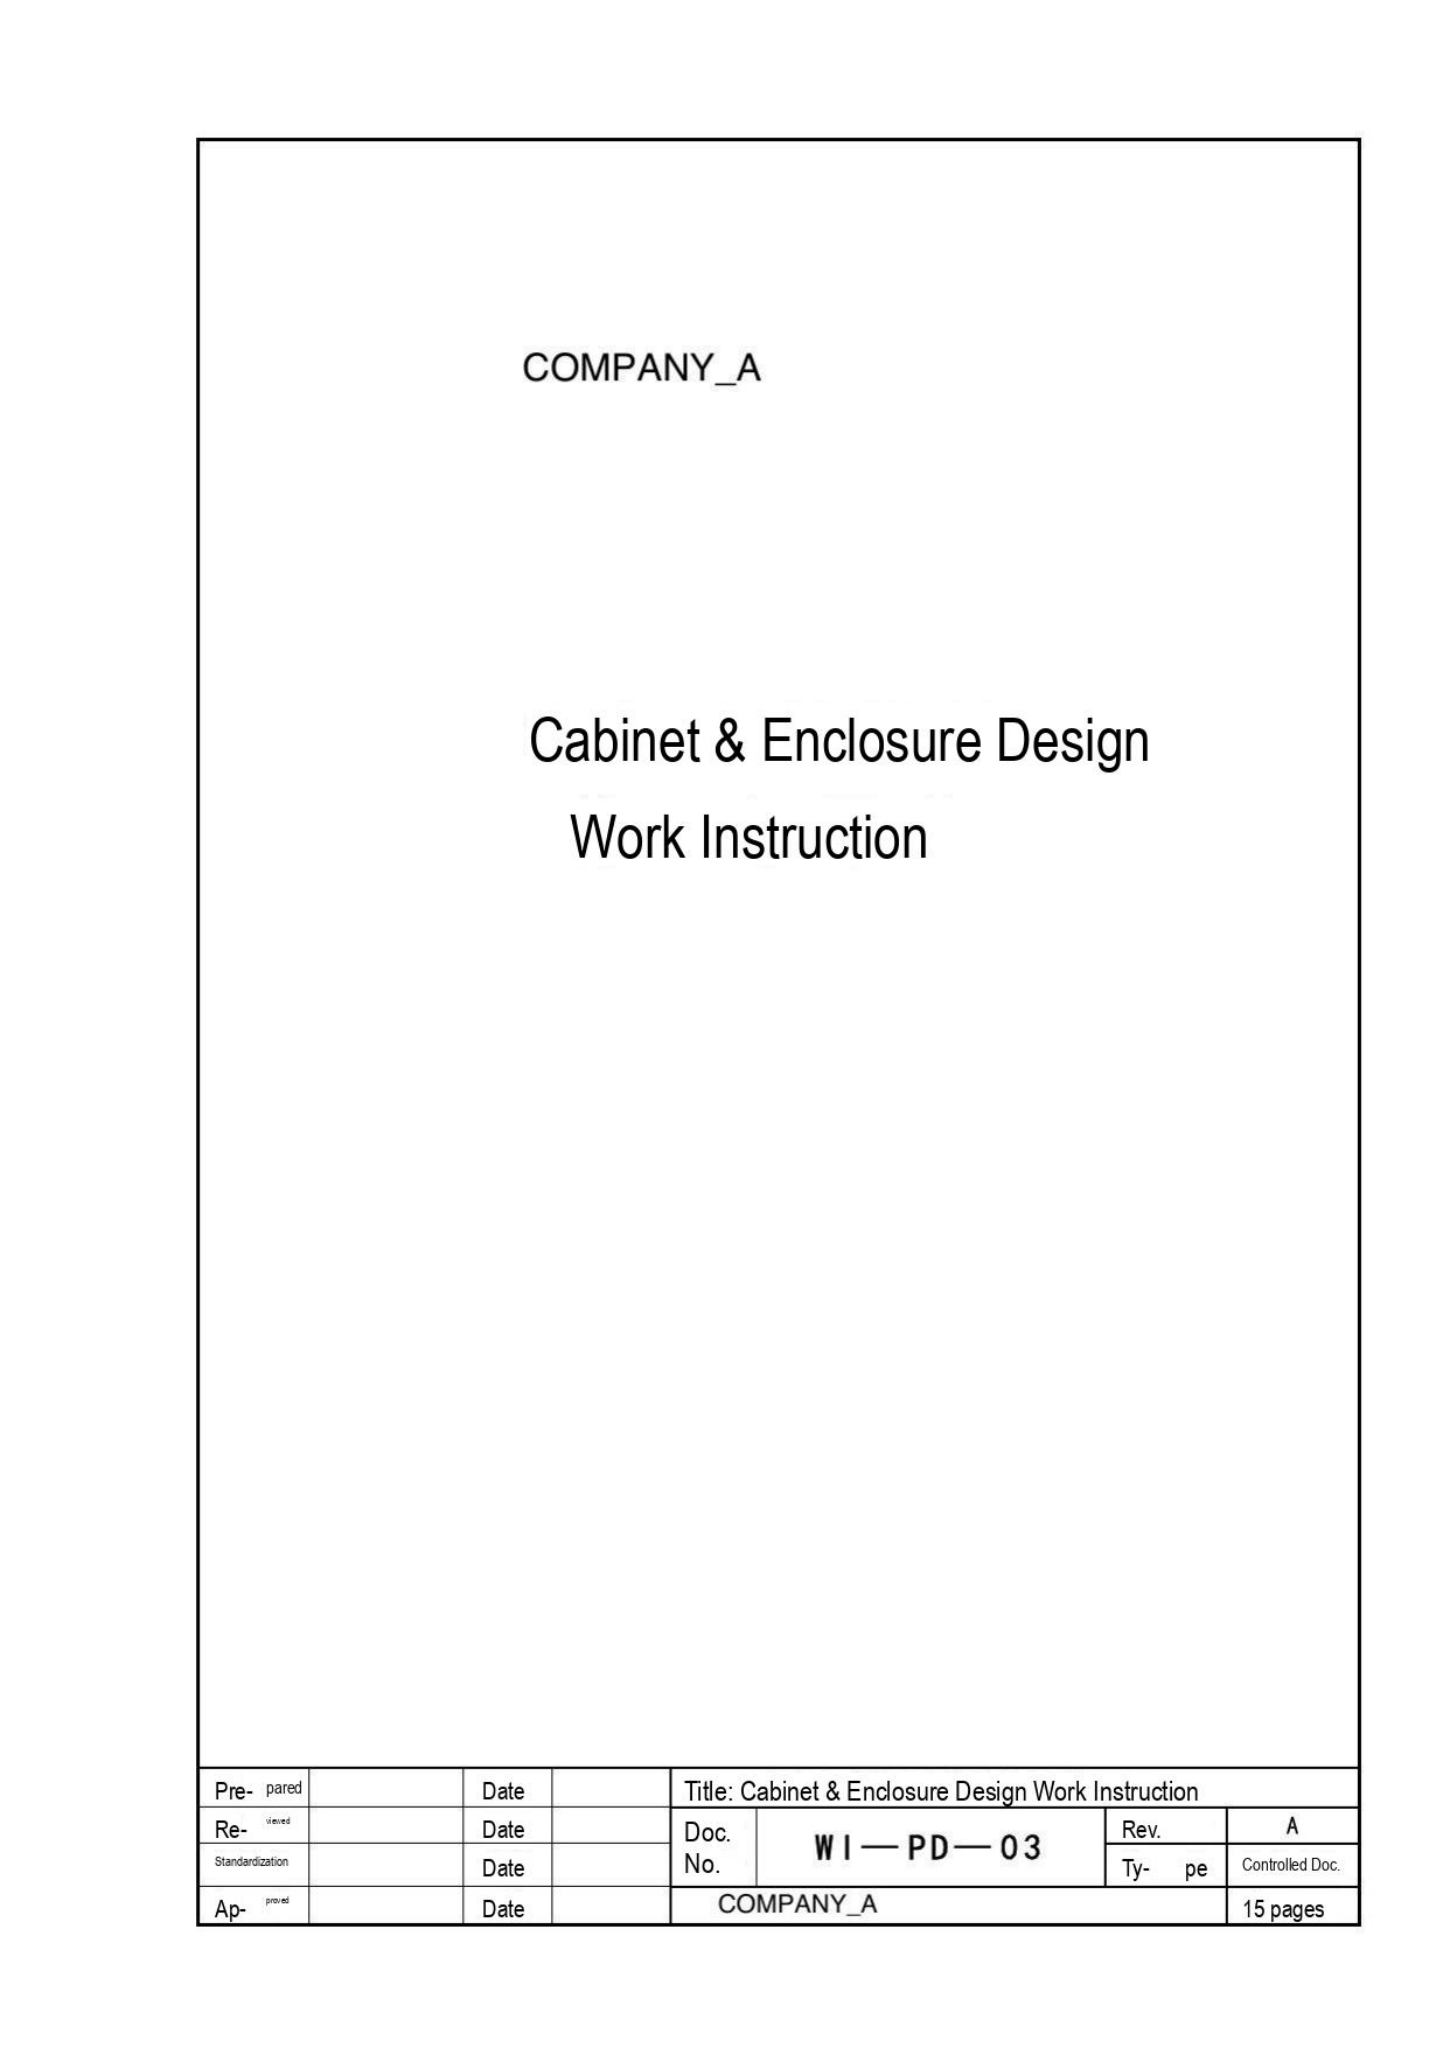COMPANY_A

Cabinet & Enclosure Design

Work Instruction

| Pre- pared | | Date | | Title: Cabinet & Enclosure Design Work Instruction | | | |
|---|---|---|---|---|---|---|---|
| Re- viewed | | Date | | Doc. No. | WI—PD—03 | Rev. | A |
| Standardization | | Date | | | | Ty- pe | Controlled Doc. |
| Ap- proved | | Date | | COMPANY_A | | | 15 pages |
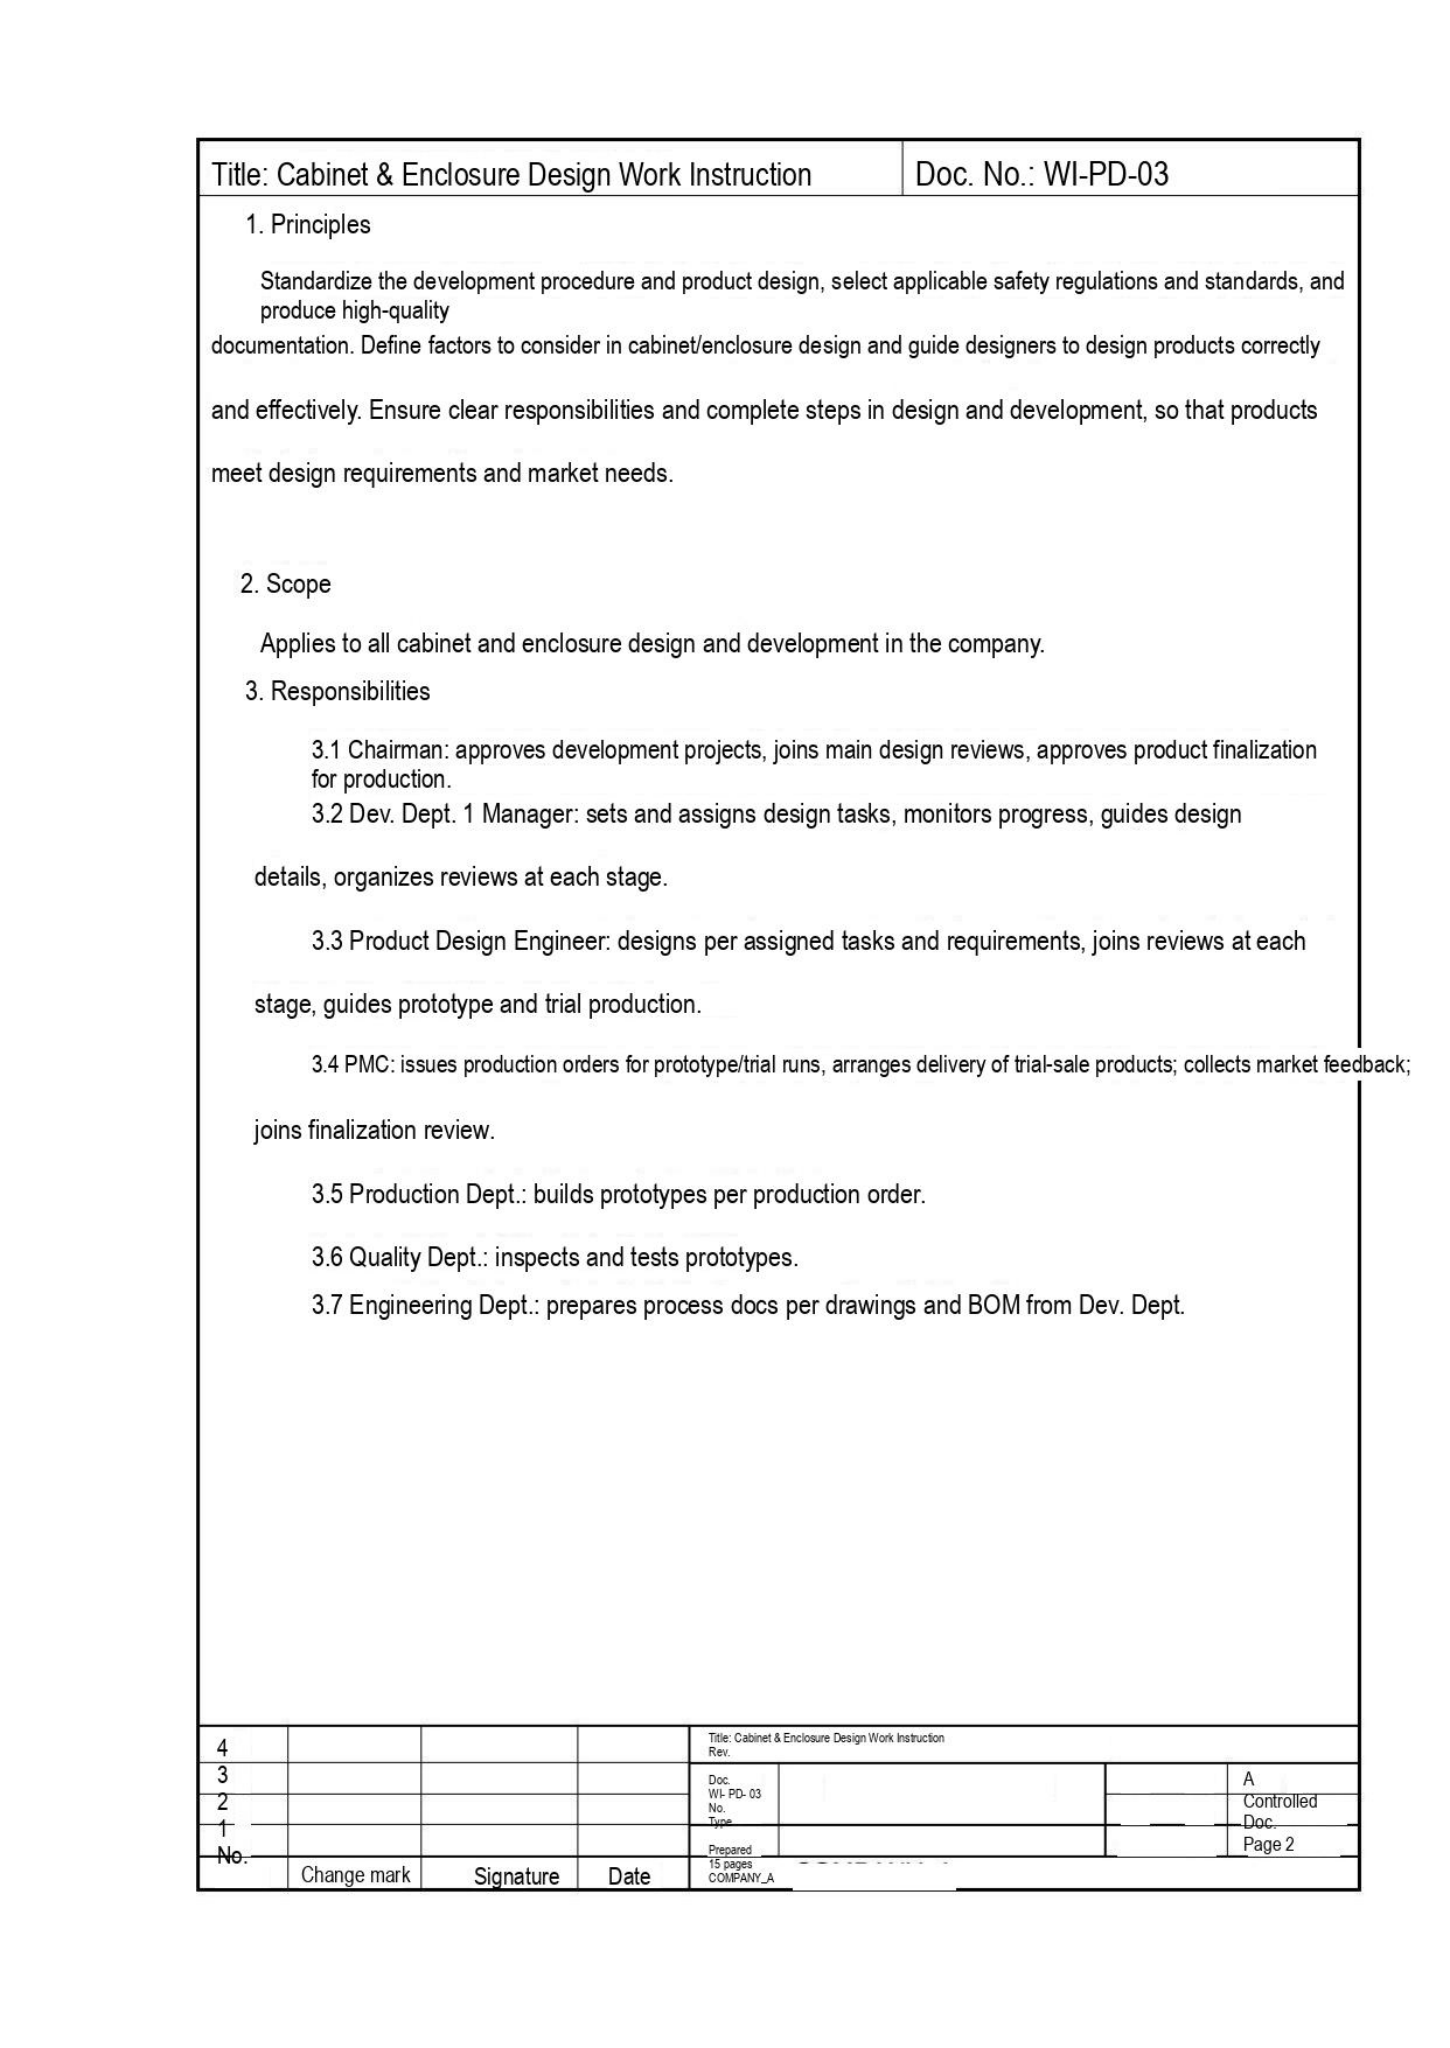Title: Cabinet & Enclosure Design Work Instruction | Doc. No.: WI-PD-03

1. Principles

Standardize the development procedure and product design, select applicable safety regulations and standards, and produce high-quality documentation. Define factors to consider in cabinet/enclosure design and guide designers to design products correctly and effectively. Ensure clear responsibilities and complete steps in design and development, so that products meet design requirements and market needs.

2. Scope

Applies to all cabinet and enclosure design and development in the company.

3. Responsibilities

3.1 Chairman: approves development projects, joins main design reviews, approves product finalization for production.

3.2 Dev. Dept. 1 Manager: sets and assigns design tasks, monitors progress, guides design details, organizes reviews at each stage.

3.3 Product Design Engineer: designs per assigned tasks and requirements, joins reviews at each stage, guides prototype and trial production.

3.4 PMC: issues production orders for prototype/trial runs, arranges delivery of trial-sale products; collects market feedback; joins finalization review.

3.5 Production Dept.: builds prototypes per production order.

3.6 Quality Dept.: inspects and tests prototypes.

3.7 Engineering Dept.: prepares process docs per drawings and BOM from Dev. Dept.

| 4 | | | | Title: Cabinet & Enclosure Design Work Instruction Rev. | | | |
|---|---|---|---|---|---|---|---|
| 3 | | | | Doc. WI- PD- 03 No. | | | A |
| 2 | | | | | | | Controlled |
| 1 | | | | Type | | | Doc. |
| No. | | | | Prepared | | | Page 2 |
| | Change mark | Signature | Date | 15 pages COMPANY_A | | | |
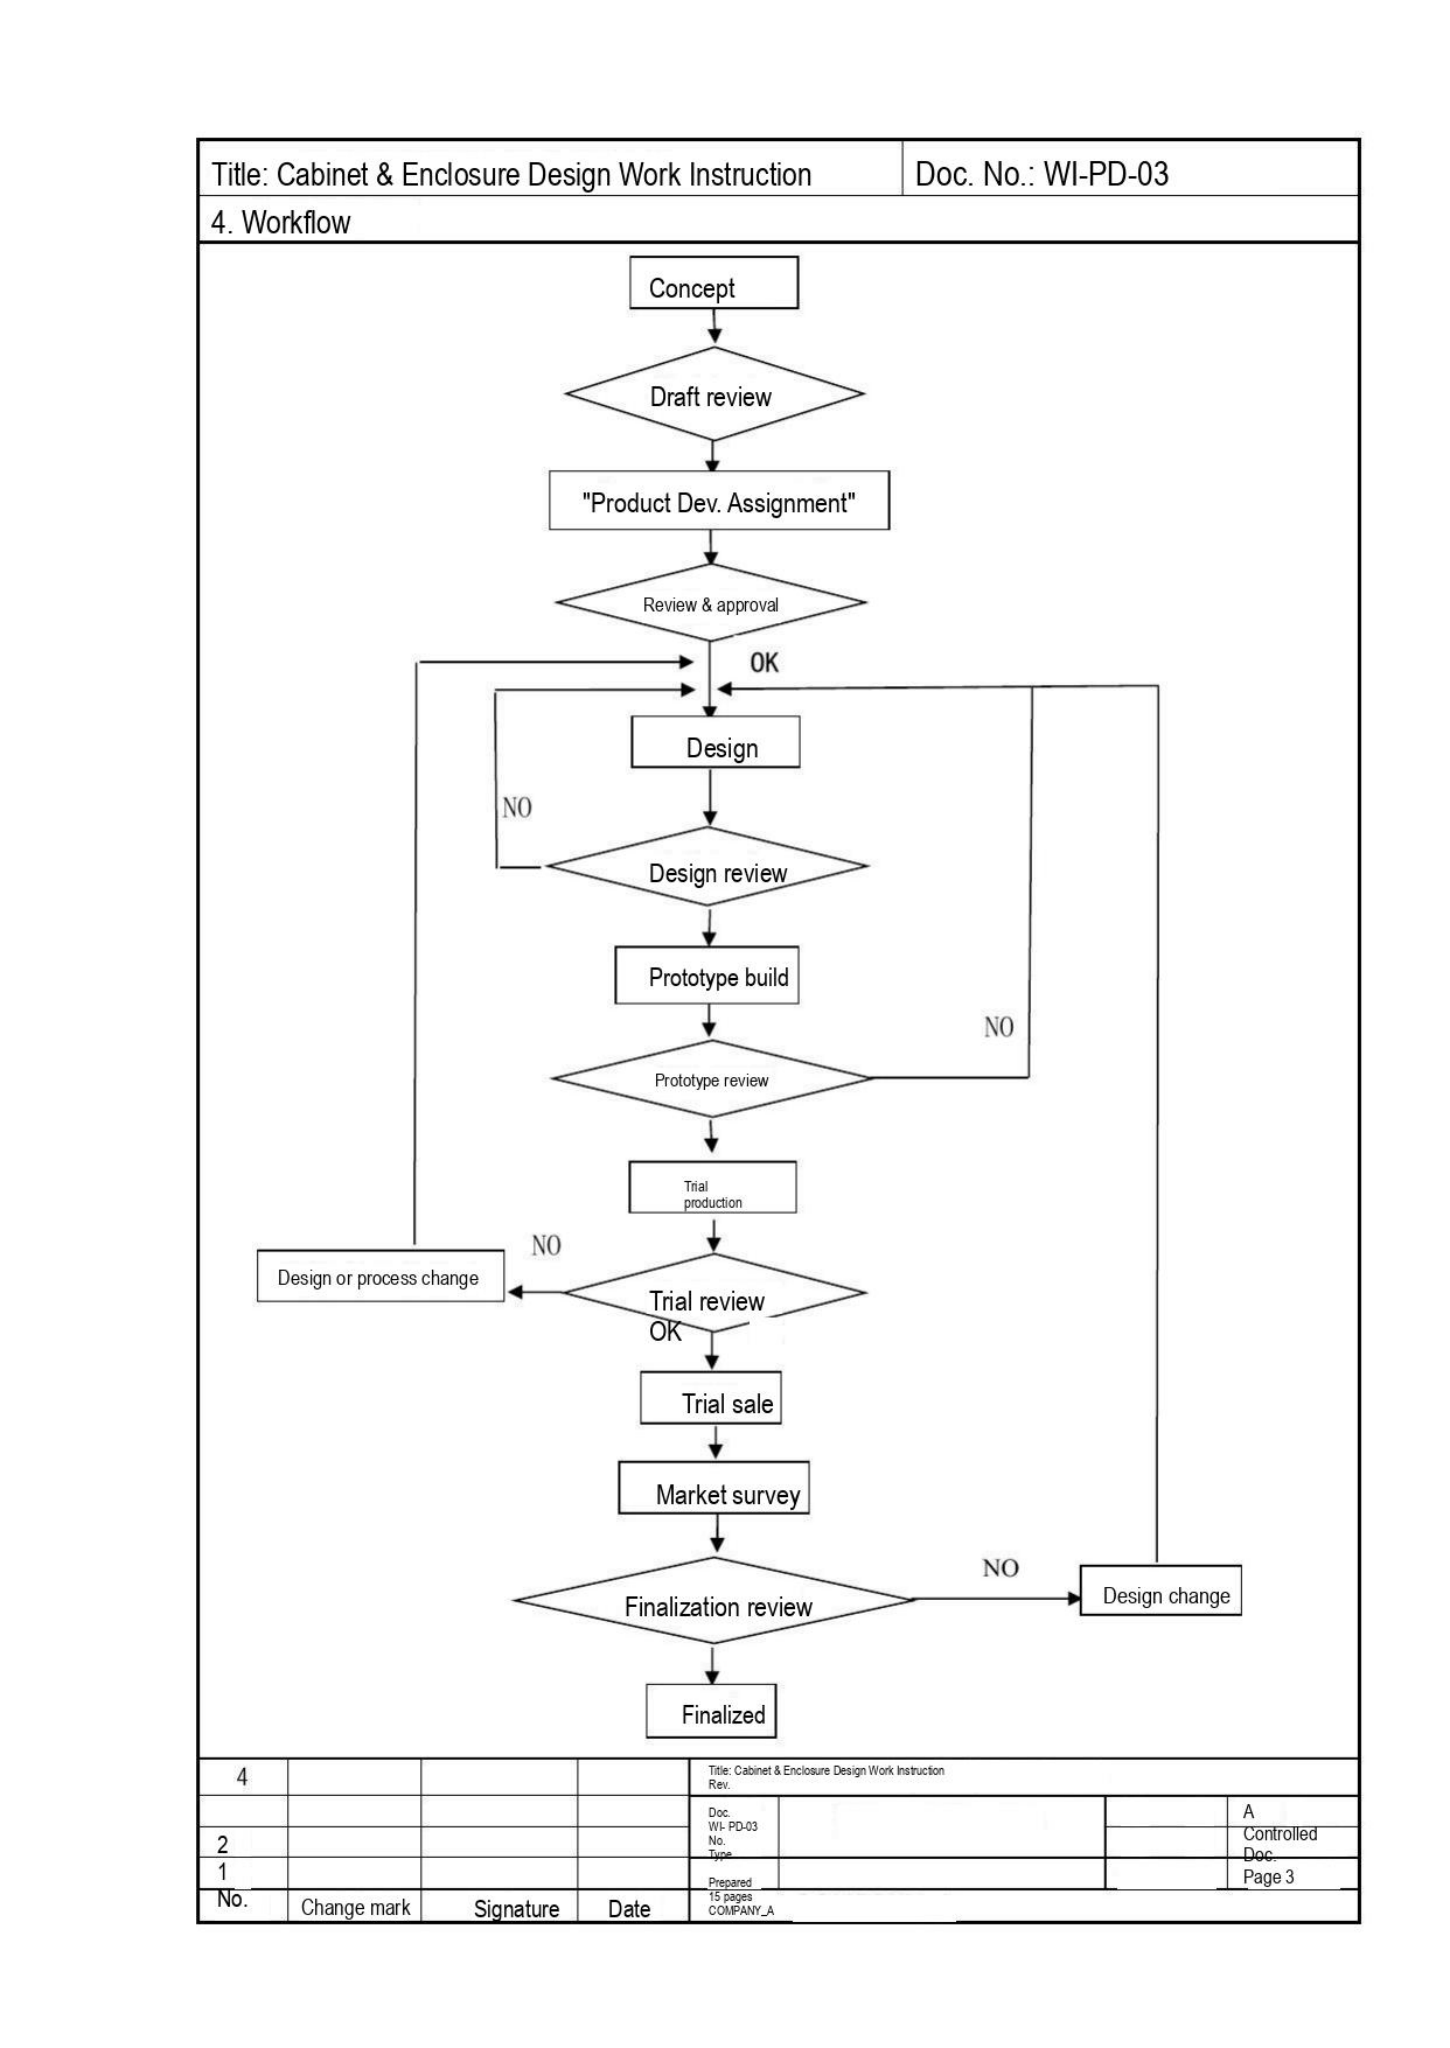Title: Cabinet & Enclosure Design Work Instruction | Doc. No.: WI-PD-03

4. Workflow

Concept

Draft review

"Product Dev. Assignment"

Review & approval

OK

Design

NO

Design review

Prototype build

NO

Prototype review

Trial production

NO

Design or process change

Trial review

OK

Trial sale

Market survey

NO

Finalization review

Design change

Finalized

| 4 | | | | Title: Cabinet & Enclosure Design Work Instruction Rev. | | | |
|---|---|---|---|---|---|---|---|
| | | | | Doc. WI- PD-03 No. Type | | | A Controlled Doc. |
| 2 | | | | | | | |
| 1 | | | | Prepared | | | Page 3 |
| No. | Change mark | Signature | Date | 15 pages COMPANY_A | | | |
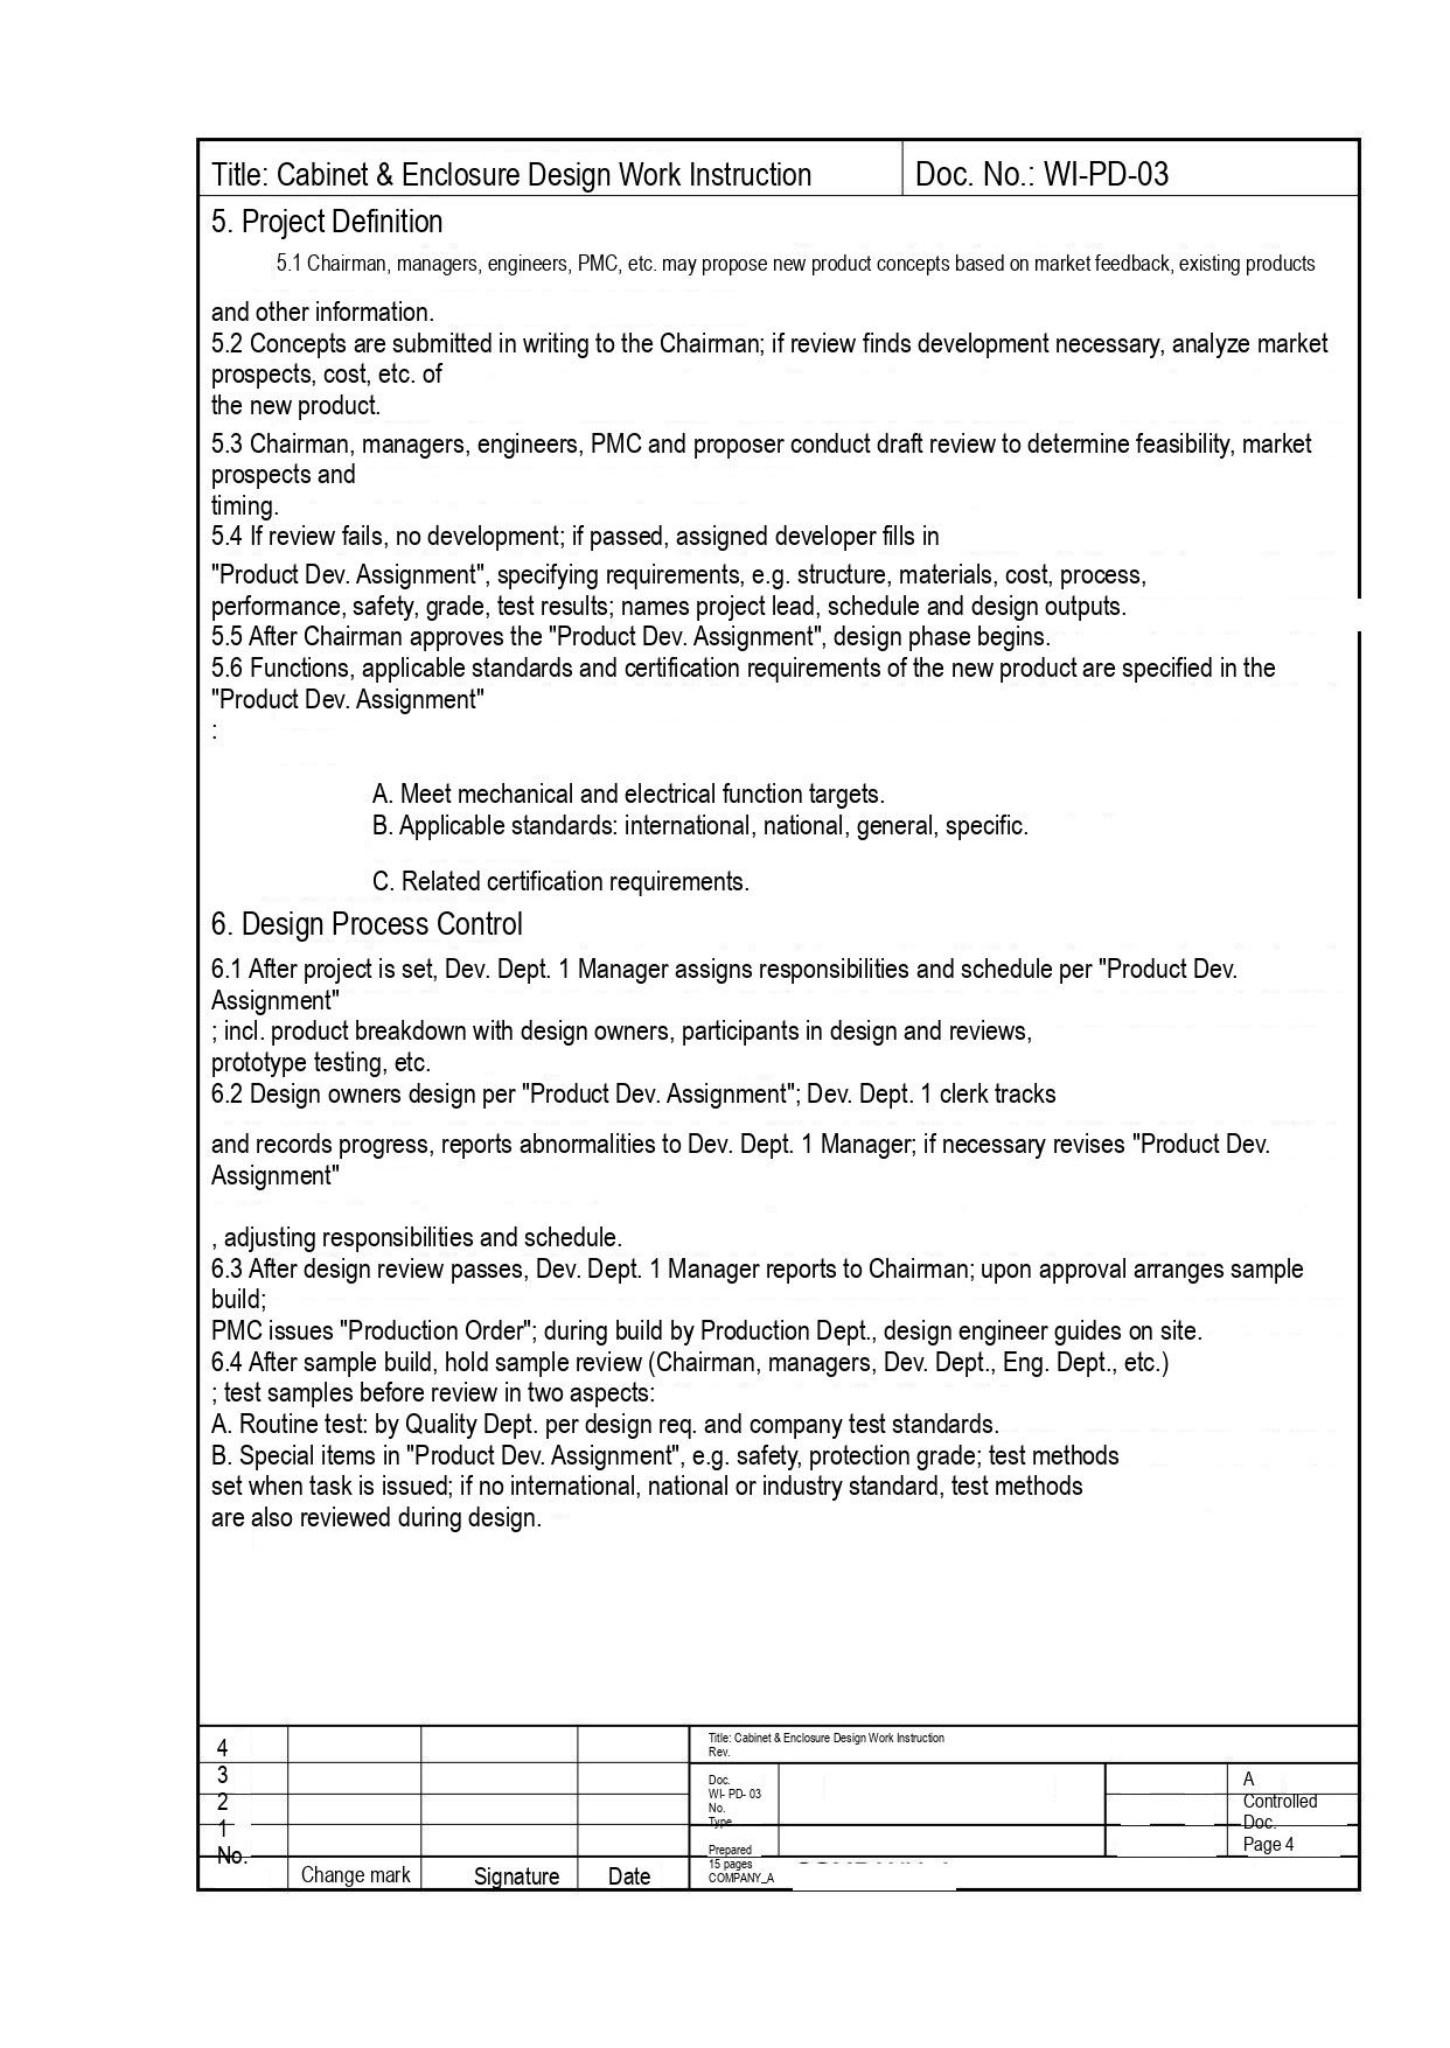| Title: Cabinet & Enclosure Design Work Instruction | Doc. No.: WI-PD-03 |
|---|---|

5. Project Definition

5.1 Chairman, managers, engineers, PMC, etc. may propose new product concepts based on market feedback, existing products and other information.

5.2 Concepts are submitted in writing to the Chairman; if review finds development necessary, analyze market prospects, cost, etc. of the new product.

5.3 Chairman, managers, engineers, PMC and proposer conduct draft review to determine feasibility, market prospects and timing.

5.4 If review fails, no development; if passed, assigned developer fills in "Product Dev. Assignment", specifying requirements, e.g. structure, materials, cost, process, performance, safety, grade, test results; names project lead, schedule and design outputs.

5.5 After Chairman approves the "Product Dev. Assignment", design phase begins.

5.6 Functions, applicable standards and certification requirements of the new product are specified in the "Product Dev. Assignment" :

A. Meet mechanical and electrical function targets.
B. Applicable standards: international, national, general, specific.
C. Related certification requirements.

6. Design Process Control

6.1 After project is set, Dev. Dept. 1 Manager assigns responsibilities and schedule per "Product Dev. Assignment" ; incl. product breakdown with design owners, participants in design and reviews, prototype testing, etc.

6.2 Design owners design per "Product Dev. Assignment"; Dev. Dept. 1 clerk tracks and records progress, reports abnormalities to Dev. Dept. 1 Manager; if necessary revises "Product Dev. Assignment" , adjusting responsibilities and schedule.

6.3 After design review passes, Dev. Dept. 1 Manager reports to Chairman; upon approval arranges sample build; PMC issues "Production Order"; during build by Production Dept., design engineer guides on site.

6.4 After sample build, hold sample review (Chairman, managers, Dev. Dept., Eng. Dept., etc.) ; test samples before review in two aspects:
A. Routine test: by Quality Dept. per design req. and company test standards.
B. Special items in "Product Dev. Assignment", e.g. safety, protection grade; test methods set when task is issued; if no international, national or industry standard, test methods are also reviewed during design.

| 4 | | | | Title: Cabinet & Enclosure Design Work Instruction Rev. | | | |
|---|---|---|---|---|---|---|---|
| 3 | | | | Doc. WI- PD- 03 No. | | | A |
| 2 | | | | Type | | | Controlled Doc. |
| 1 | | | | Prepared | | | Page 4 |
| No. | Change mark | Signature | Date | 15 pages COMPANY_A | | | |
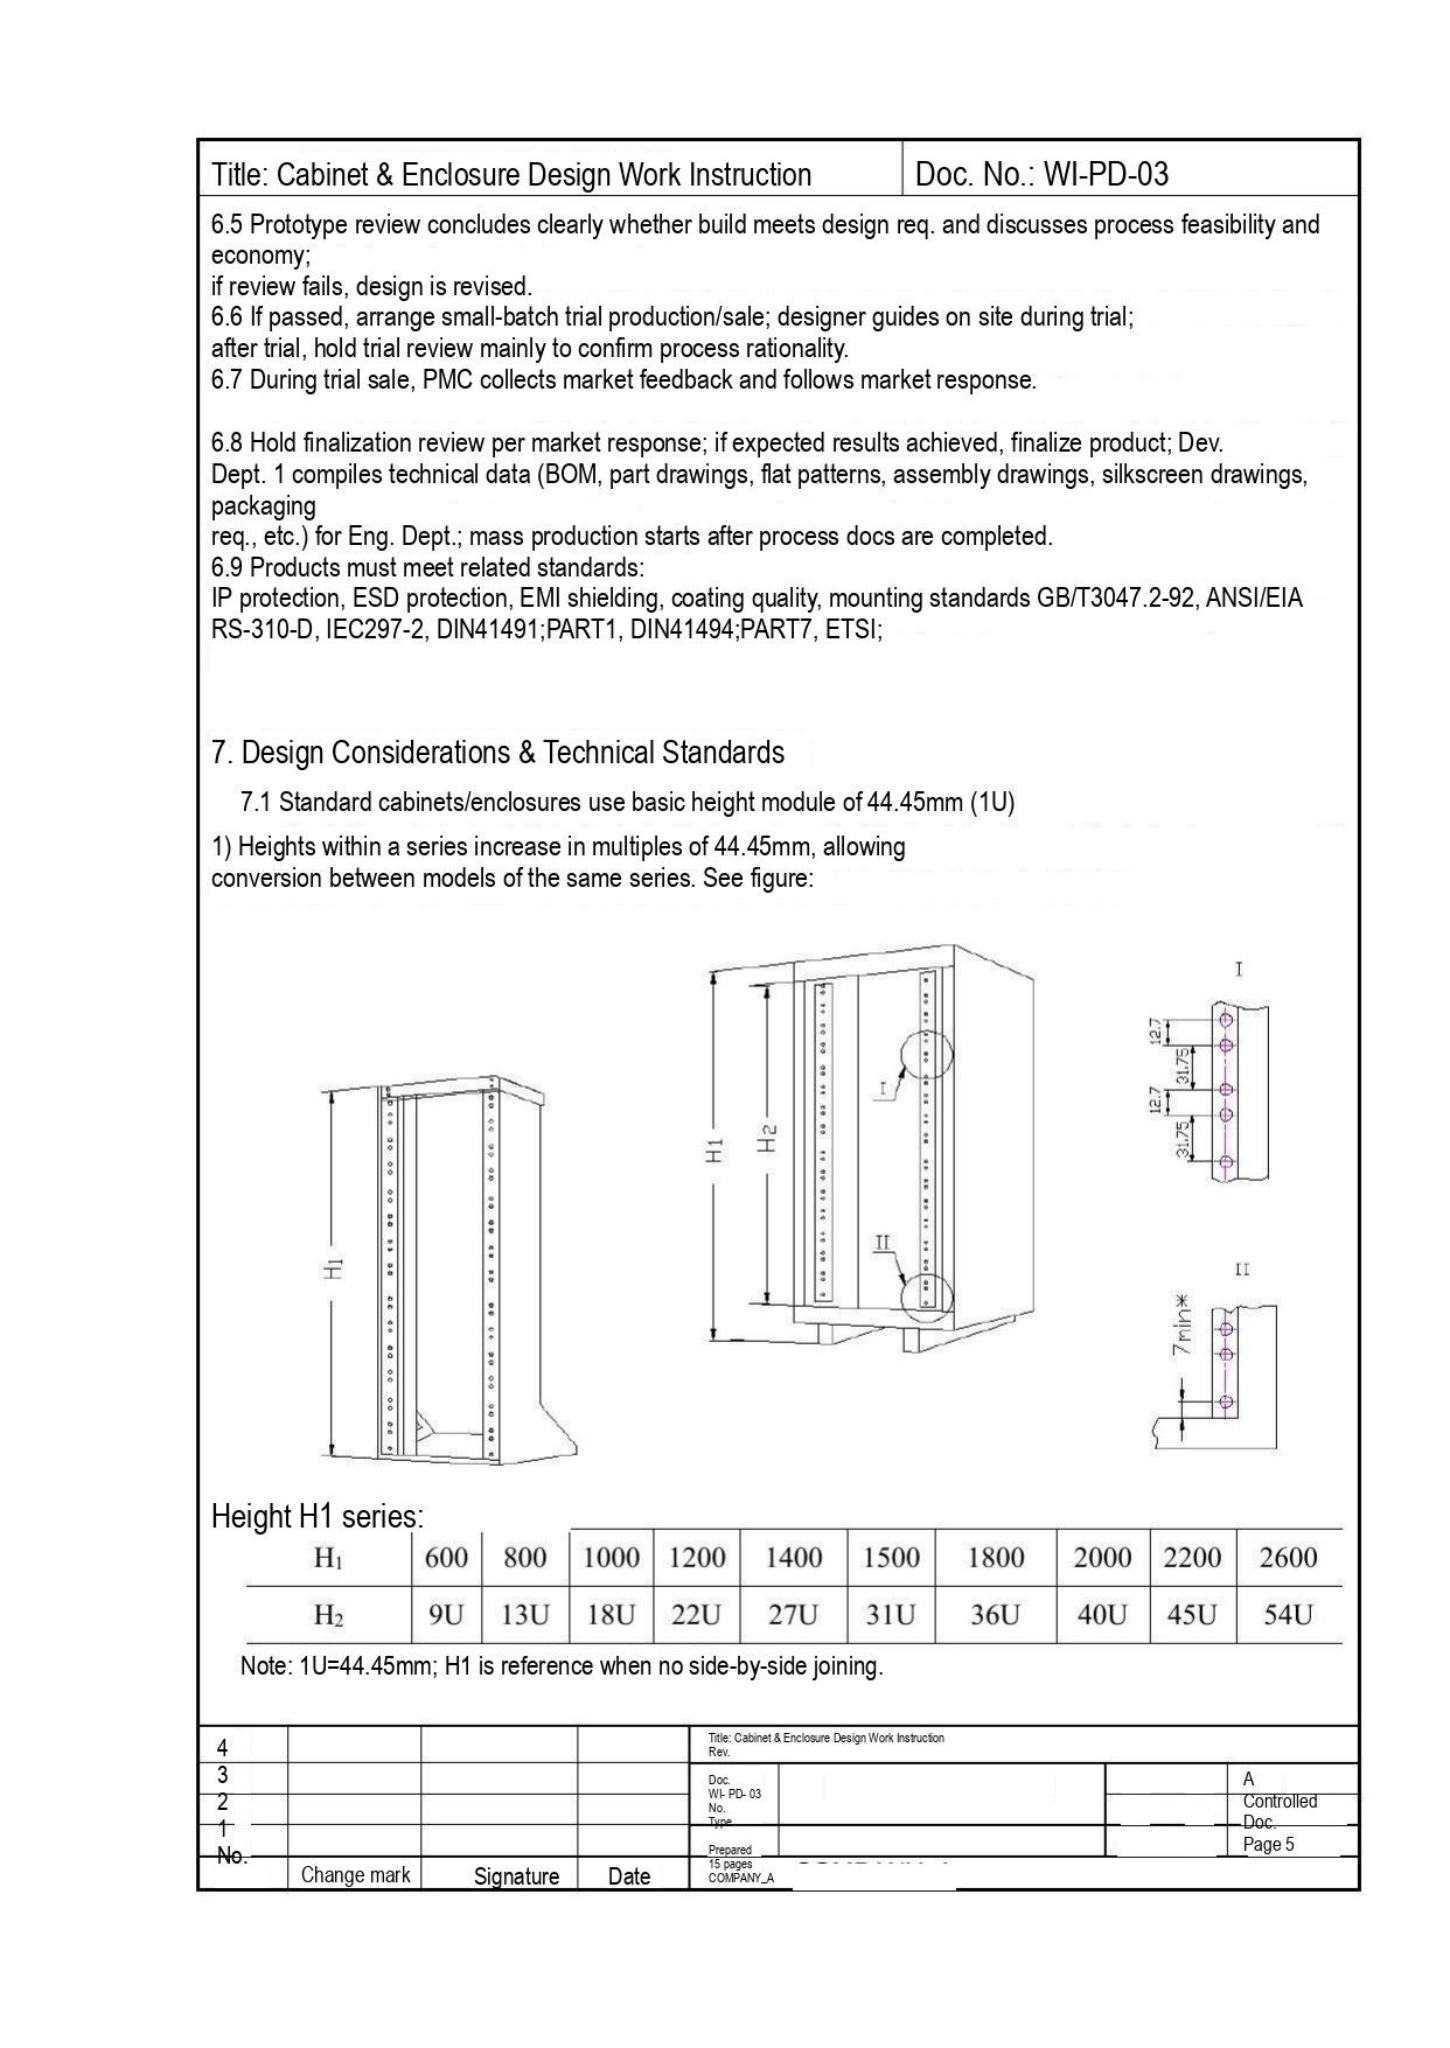| Title: Cabinet & Enclosure Design Work Instruction | Doc. No.: WI-PD-03 |
|---|---|

6.5 Prototype review concludes clearly whether build meets design req. and discusses process feasibility and economy;
if review fails, design is revised.
6.6 If passed, arrange small-batch trial production/sale; designer guides on site during trial;
after trial, hold trial review mainly to confirm process rationality.
6.7 During trial sale, PMC collects market feedback and follows market response.

6.8 Hold finalization review per market response; if expected results achieved, finalize product; Dev.
Dept. 1 compiles technical data (BOM, part drawings, flat patterns, assembly drawings, silkscreen drawings, packaging
req., etc.) for Eng. Dept.; mass production starts after process docs are completed.
6.9 Products must meet related standards:
IP protection, ESD protection, EMI shielding, coating quality, mounting standards GB/T3047.2-92, ANSI/EIA RS-310-D, IEC297-2, DIN41491;PART1, DIN41494;PART7, ETSI;

7. Design Considerations & Technical Standards

7.1 Standard cabinets/enclosures use basic height module of 44.45mm (1U)

1) Heights within a series increase in multiples of 44.45mm, allowing
conversion between models of the same series. See figure:

H1

H1 H2 I II

I
12.7 31.75 12.7 31.75

II
7min*

Height H1 series:

| H₁ | 600 | 800 | 1000 | 1200 | 1400 | 1500 | 1800 | 2000 | 2200 | 2600 |
|---|---|---|---|---|---|---|---|---|---|---|
| H₂ | 9U | 13U | 18U | 22U | 27U | 31U | 36U | 40U | 45U | 54U |

Note: 1U=44.45mm; H1 is reference when no side-by-side joining.

| 4 | | | | Title: Cabinet & Enclosure Design Work Instruction Rev. | | | |
|---|---|---|---|---|---|---|---|
| 3 | | | | Doc. WI- PD- 03 No. | | | A |
| 2 | | | | | | | Controlled Doc. |
| 1 | | | | Type | | | |
| No. | | | | Prepared | | | Page 5 |
| | Change mark | Signature | Date | 15 pages COMPANY_A | | | |
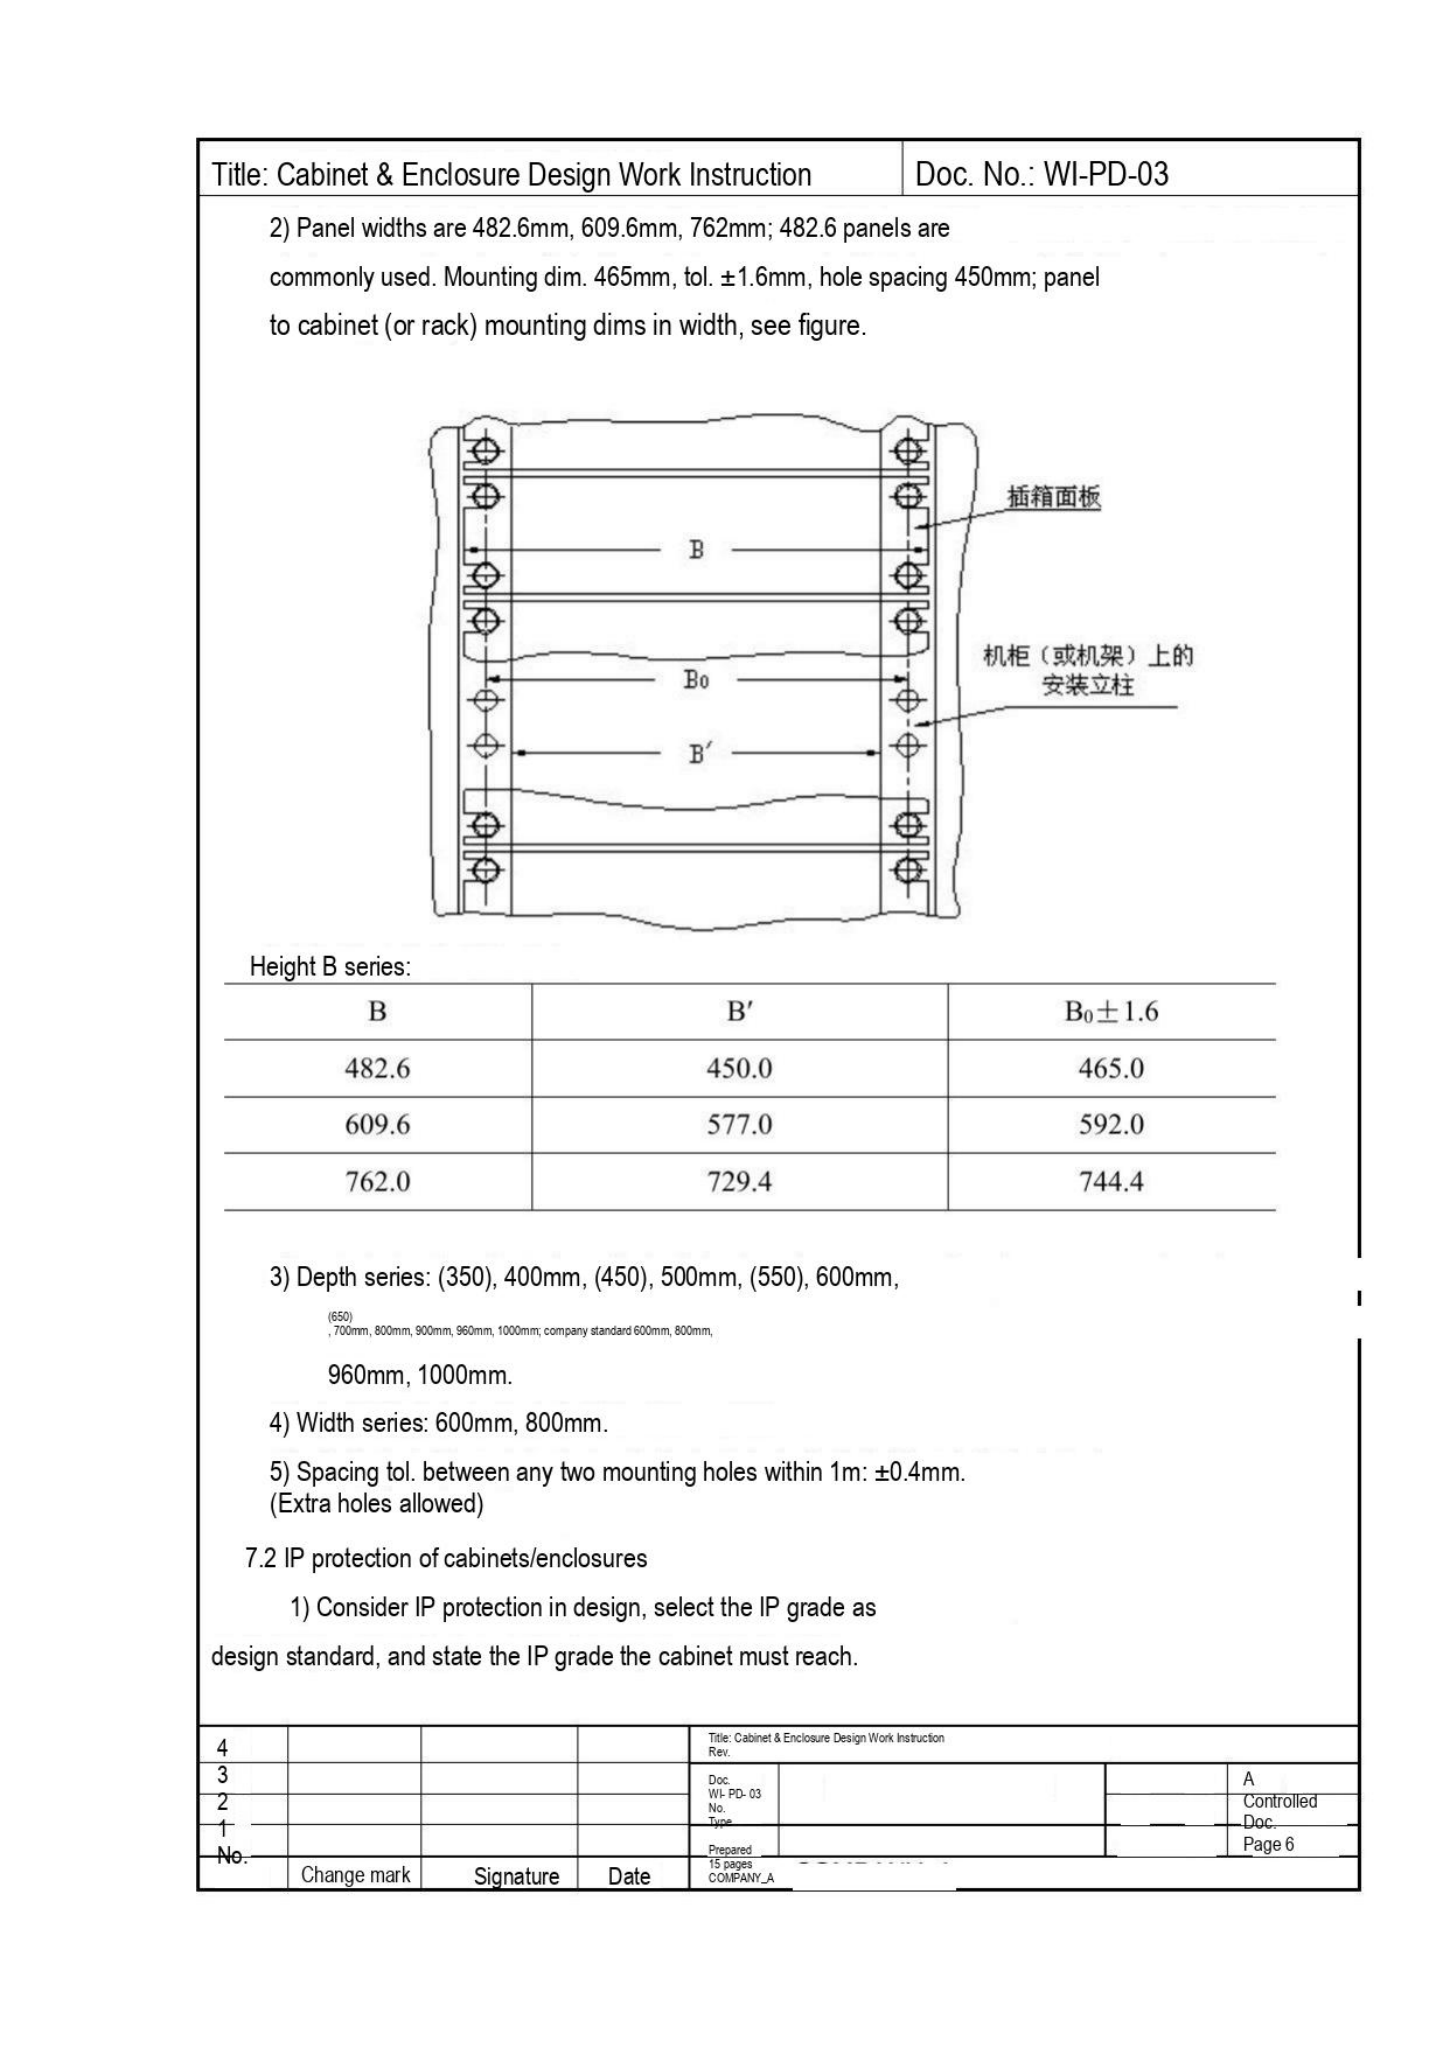| Title: Cabinet & Enclosure Design Work Instruction | Doc. No.: WI-PD-03 |
|---|---|

2) Panel widths are 482.6mm, 609.6mm, 762mm; 482.6 panels are commonly used. Mounting dim. 465mm, tol. ±1.6mm, hole spacing 450mm; panel to cabinet (or rack) mounting dims in width, see figure.

B

插箱面板

B₀

机柜（或机架）上的
安装立柱

B′

Height B series:

| B | B′ | B₀±1.6 |
|---|---|---|
| 482.6 | 450.0 | 465.0 |
| 609.6 | 577.0 | 592.0 |
| 762.0 | 729.4 | 744.4 |

3) Depth series: (350), 400mm, (450), 500mm, (550), 600mm,

(650)
, 700mm, 800mm, 900mm, 960mm, 1000mm; company standard 600mm, 800mm,

960mm, 1000mm.

4) Width series: 600mm, 800mm.

5) Spacing tol. between any two mounting holes within 1m: ±0.4mm.
(Extra holes allowed)

7.2 IP protection of cabinets/enclosures

1) Consider IP protection in design, select the IP grade as design standard, and state the IP grade the cabinet must reach.

| 4 | | | | Title: Cabinet & Enclosure Design Work Instruction<br>Rev. | | | |
|---|---|---|---|---|---|---|---|
| 3 | | | | Doc.<br>WI- PD- 03<br>No.<br>Type | | | A<br>Controlled<br>Doc. |
| 2 | | | | | | | |
| 1 | | | | Prepared | | | Page 6 |
| No. | Change mark | Signature | Date | 15 pages<br>COMPANY_A | | | |
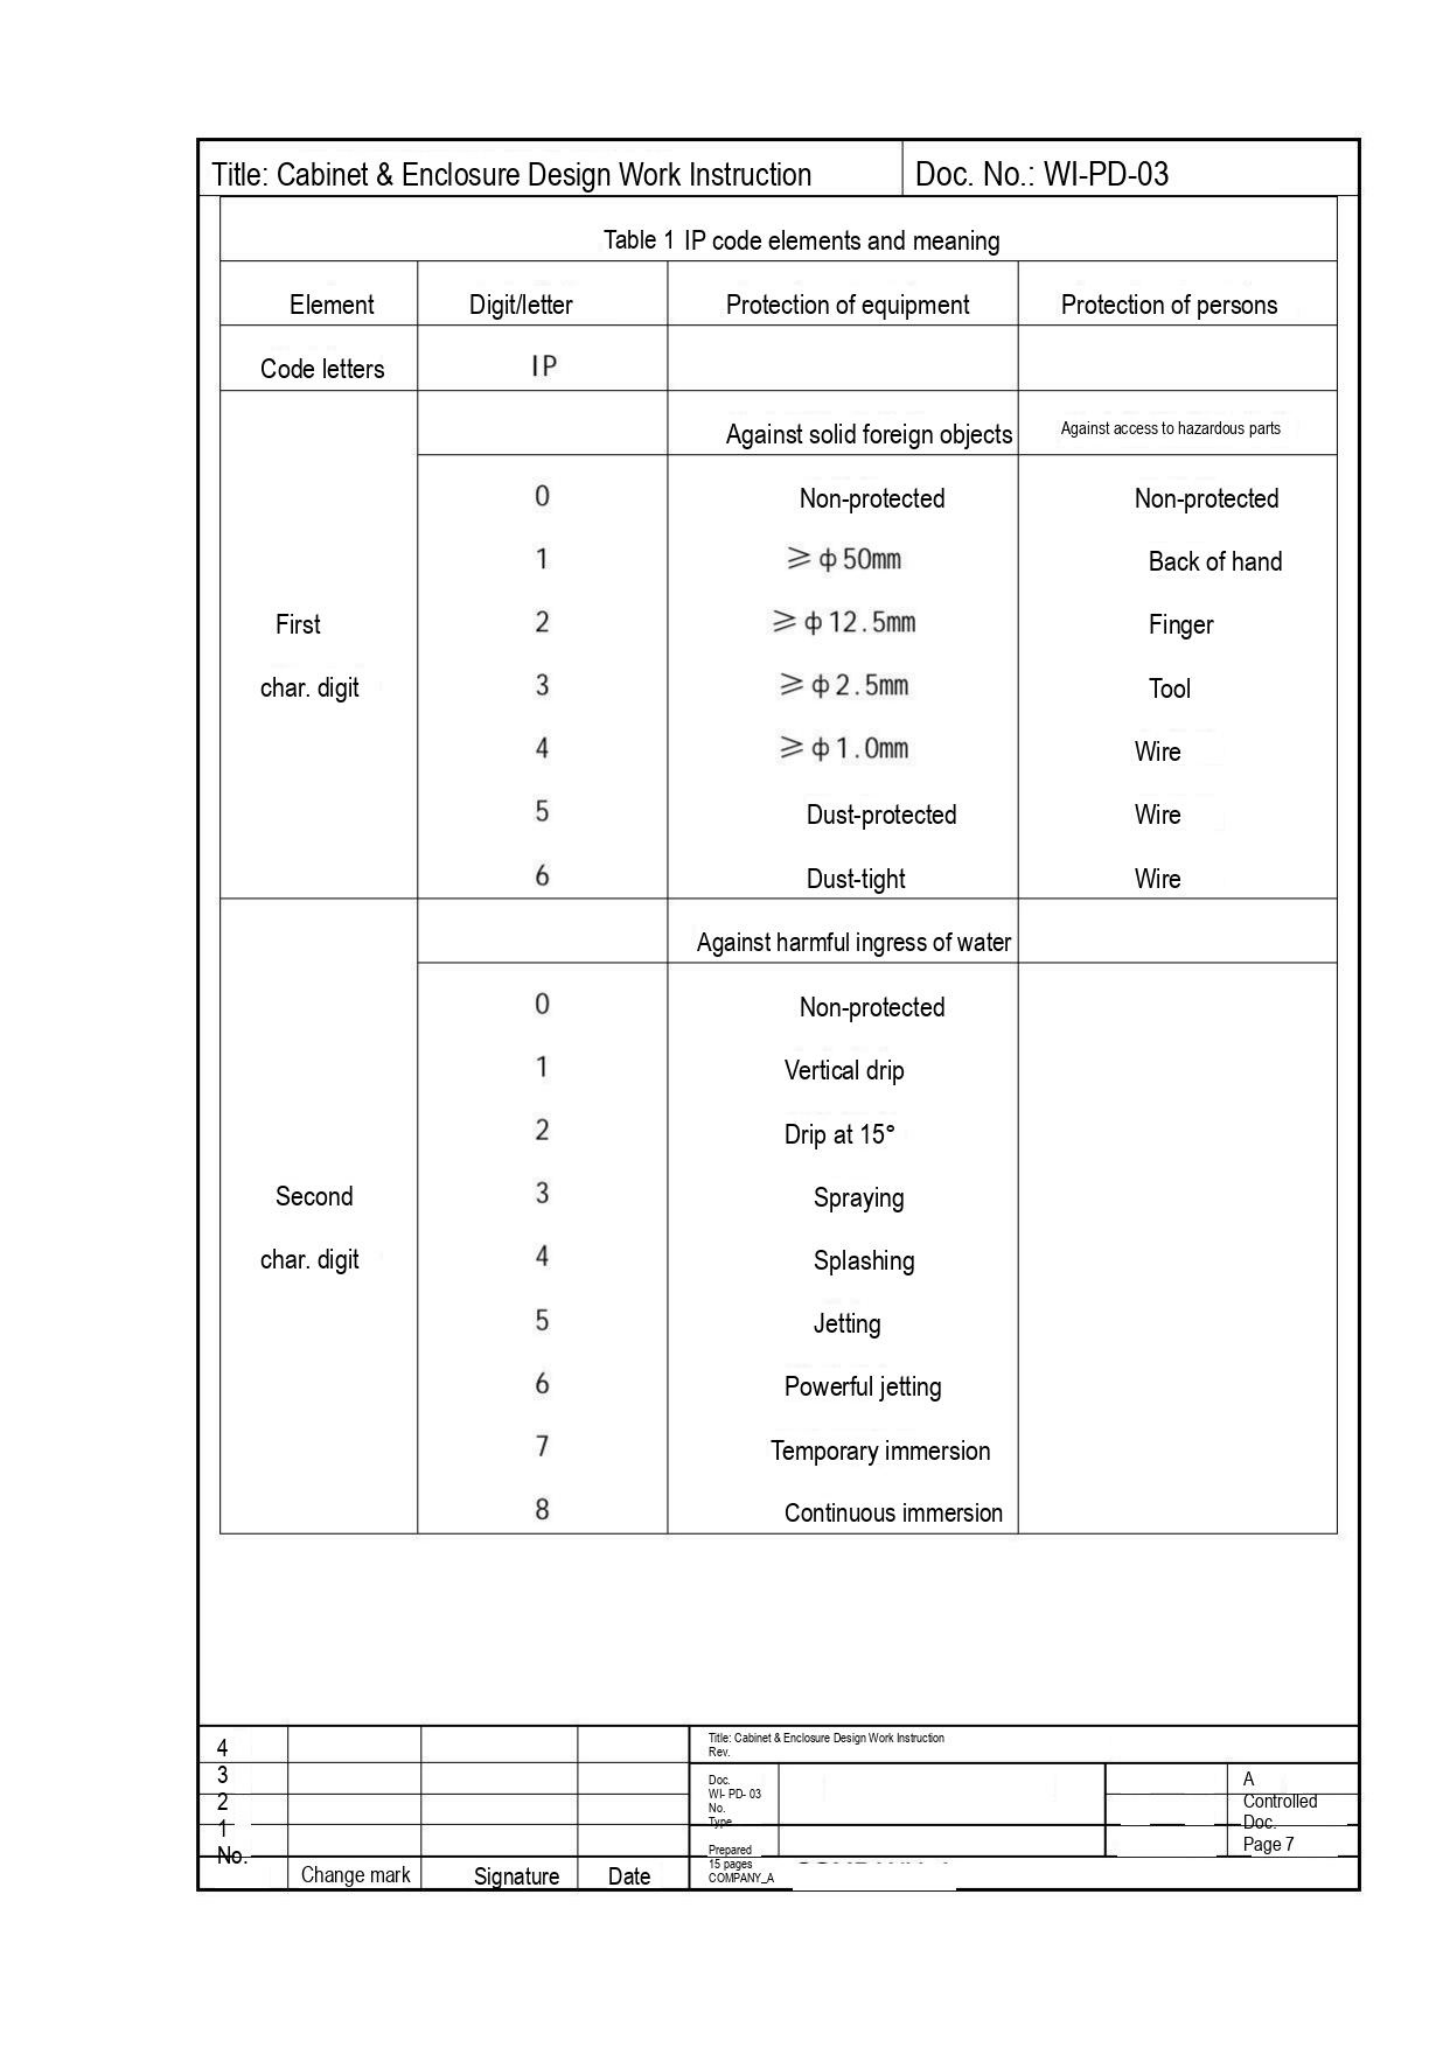Title: Cabinet & Enclosure Design Work Instruction | Doc. No.: WI-PD-03

Table 1 IP code elements and meaning

| Element | Digit/letter | Protection of equipment | Protection of persons |
|---|---|---|---|
| Code letters | IP | | |
| First char. digit | | Against solid foreign objects | Against access to hazardous parts |
| | 0 | Non-protected | Non-protected |
| | 1 | ≥ φ 50mm | Back of hand |
| | 2 | ≥ φ 12.5mm | Finger |
| | 3 | ≥ φ 2.5mm | Tool |
| | 4 | ≥ φ 1.0mm | Wire |
| | 5 | Dust-protected | Wire |
| | 6 | Dust-tight | Wire |
| Second char. digit | | Against harmful ingress of water | |
| | 0 | Non-protected | |
| | 1 | Vertical drip | |
| | 2 | Drip at 15° | |
| | 3 | Spraying | |
| | 4 | Splashing | |
| | 5 | Jetting | |
| | 6 | Powerful jetting | |
| | 7 | Temporary immersion | |
| | 8 | Continuous immersion | |

| No. | Change mark | Signature | Date |
|---|---|---|---|
| 4 | | | |
| 3 | | | |
| 2 | | | |
| 1 | | | |

Title: Cabinet & Enclosure Design Work Instruction
Rev.
Doc. No.: WI- PD- 03
Type
Prepared
15 pages
COMPANY_A
A
Controlled Doc.
Page 7